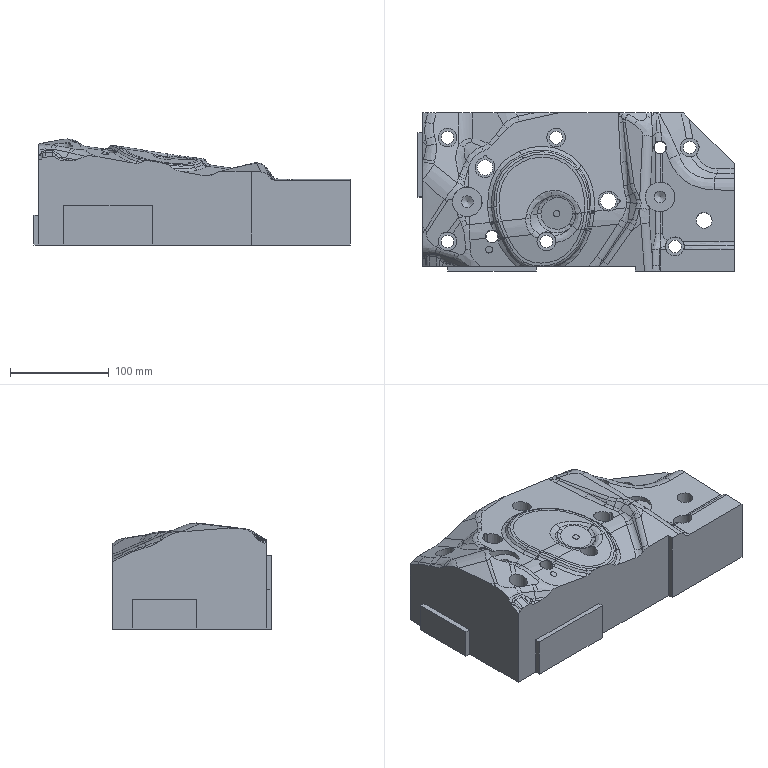Part | NX | features solid 2 | 1 solid | 317 faces | box 320 x 160.091 x 107.263 mm | volume 3713532 mm3 | spline 156 | cylinder 93 | plane 61 | cone 6 | sphere 1 | commonest cylinder face diameters 16 x14 13 x8 19 x6 20 x5 6.001 x4 12 x4